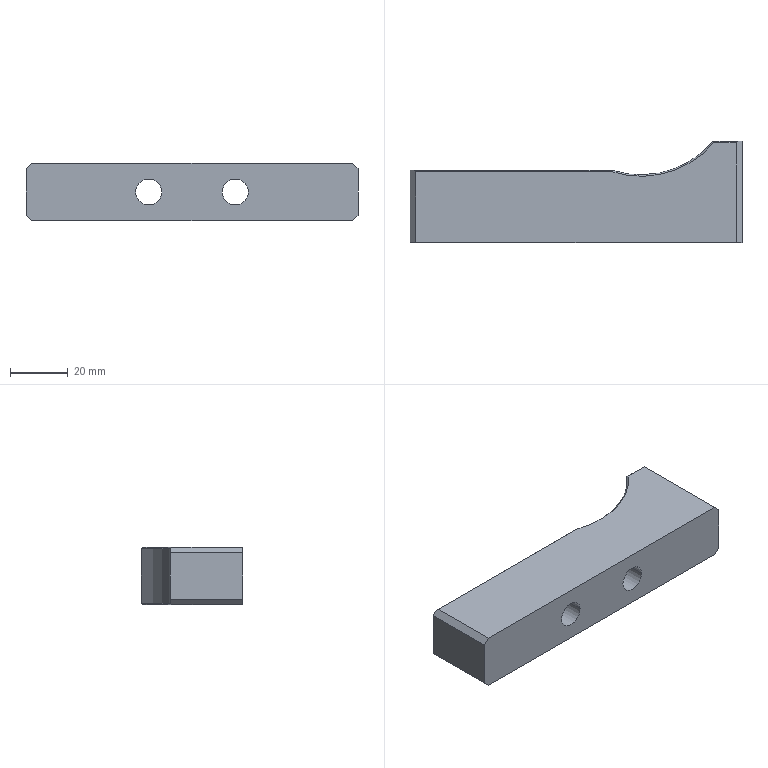Part | SolidWorks | features Chamfer 2, ICE 2, Extrusion 1 | 1 solid | 28 faces | box 115 x 35 x 20 mm | volume 55138 mm3 | plane 17 | cylinder 9 | cone 2 | commonest cylinder face diameters 9 x4 14 x4 65 x1
STEP:
#1=CARTESIAN_POINT('',(77.,0.,10.));
#2=VERTEX_POINT('',#1);
#3=CARTESIAN_POINT('',(68.,0.,10.));
#4=VERTEX_POINT('',#3);
#5=CARTESIAN_POINT('',(72.5,0.,10.));
#6=DIRECTION('',(0.,1.,0.));
#7=DIRECTION('',(-1.,0.,0.));
#8=AXIS2_PLACEMENT_3D('',#5,#6,#7);
#9=CIRCLE('',#8,4.5);
#10=EDGE_CURVE('',#2,#4,#9,.T.);
#11=ORIENTED_EDGE('',*,*,#10,.F.);
#12=CARTESIAN_POINT('',(77.,15.,10.));
#13=VERTEX_POINT('',#12);
#14=CARTESIAN_POINT('',(77.,-5.,10.));
#15=DIRECTION('',(0.,1.,0.));
#16=VECTOR('',#15,1000.);
#17=LINE('',#14,#16);
#18=EDGE_CURVE('',#2,#13,#17,.T.);
#19=ORIENTED_EDGE('',*,*,#18,.T.);
#20=CARTESIAN_POINT('',(68.,15.,10.));
#21=VERTEX_POINT('',#20);
#22=CARTESIAN_POINT('',(72.5,15.,10.));
#23=DIRECTION('',(0.,1.,0.));
#24=DIRECTION('',(-1.,0.,0.));
#25=AXIS2_PLACEMENT_3D('',#22,#23,#24);
#26=CIRCLE('',#25,4.5);
#27=EDGE_CURVE('',#13,#21,#26,.T.);
#28=ORIENTED_EDGE('',*,*,#27,.T.);
#29=CARTESIAN_POINT('',(68.,-5.,10.));
#30=DIRECTION('',(0.,1.,0.));
#31=VECTOR('',#30,1000.);
#32=LINE('',#29,#31);
#33=EDGE_CURVE('',#4,#21,#32,.T.);
#34=ORIENTED_EDGE('',*,*,#33,.F.);
#35=EDGE_LOOP('',(#11,#19,#28,#34));
#36=FACE_OUTER_BOUND('',#35,.T.);
#37=CARTESIAN_POINT('',(72.5,-5.,10.));
#38=DIRECTION('',(0.,1.,0.));
#39=DIRECTION('',(-1.,0.,0.));
#40=AXIS2_PLACEMENT_3D('',#37,#38,#39);
#41=CYLINDRICAL_SURFACE('',#40,4.5);
#42=ADVANCED_FACE('',(#36),#41,.F.);
#43=CARTESIAN_POINT('',(47.,0.,10.));
#44=VERTEX_POINT('',#43);
#45=CARTESIAN_POINT('',(38.,0.,10.));
#46=VERTEX_POINT('',#45);
#47=CARTESIAN_POINT('',(42.5,0.,10.));
#48=DIRECTION('',(0.,1.,0.));
#49=DIRECTION('',(-1.,0.,0.));
#50=AXIS2_PLACEMENT_3D('',#47,#48,#49);
#51=CIRCLE('',#50,4.5);
#52=EDGE_CURVE('',#44,#46,#51,.T.);
#53=ORIENTED_EDGE('',*,*,#52,.F.);
#54=CARTESIAN_POINT('',(47.,15.,10.));
#55=VERTEX_POINT('',#54);
#56=CARTESIAN_POINT('',(47.,-5.,10.));
#57=DIRECTION('',(0.,1.,0.));
#58=VECTOR('',#57,1000.);
#59=LINE('',#56,#58);
#60=EDGE_CURVE('',#44,#55,#59,.T.);
#61=ORIENTED_EDGE('',*,*,#60,.T.);
#62=CARTESIAN_POINT('',(38.,15.,10.));
#63=VERTEX_POINT('',#62);
#64=CARTESIAN_POINT('',(42.5,15.,10.));
#65=DIRECTION('',(0.,1.,0.));
#66=DIRECTION('',(-1.,0.,0.));
#67=AXIS2_PLACEMENT_3D('',#64,#65,#66);
#68=CIRCLE('',#67,4.5);
#69=EDGE_CURVE('',#55,#63,#68,.T.);
#70=ORIENTED_EDGE('',*,*,#69,.T.);
#71=CARTESIAN_POINT('',(38.,-5.,10.));
#72=DIRECTION('',(0.,1.,0.));
#73=VECTOR('',#72,1000.);
#74=LINE('',#71,#73);
#75=EDGE_CURVE('',#46,#63,#74,.T.);
#76=ORIENTED_EDGE('',*,*,#75,.F.);
#77=EDGE_LOOP('',(#53,#61,#70,#76));
#78=FACE_OUTER_BOUND('',#77,.T.);
#79=CARTESIAN_POINT('',(42.5,-5.,10.));
#80=DIRECTION('',(0.,1.,0.));
#81=DIRECTION('',(-1.,0.,0.));
#82=AXIS2_PLACEMENT_3D('',#79,#80,#81);
#83=CYLINDRICAL_SURFACE('',#82,4.5);
#84=ADVANCED_FACE('',(#78),#83,.F.);
#85=CARTESIAN_POINT('',(79.5,15.,10.));
#86=VERTEX_POINT('',#85);
#87=CARTESIAN_POINT('',(65.5,15.,10.));
#88=VERTEX_POINT('',#87);
#89=CARTESIAN_POINT('',(72.5,15.,10.));
#90=DIRECTION('',(0.,1.,0.));
#91=DIRECTION('',(-1.,0.,0.));
#92=AXIS2_PLACEMENT_3D('',#89,#90,#91);
#93=CIRCLE('',#92,7.);
#94=EDGE_CURVE('',#86,#88,#93,.T.);
#95=ORIENTED_EDGE('',*,*,#94,.F.);
#96=CARTESIAN_POINT('',(79.5,23.427,10.));
#97=VERTEX_POINT('',#96);
#98=CARTESIAN_POINT('',(79.5,15.,10.));
#99=DIRECTION('',(0.,1.,0.));
#100=VECTOR('',#99,1000.);
#101=LINE('',#98,#100);
#102=EDGE_CURVE('',#86,#97,#101,.T.);
#103=ORIENTED_EDGE('',*,*,#102,.T.);
#104=CARTESIAN_POINT('',(70.,25.,3.462));
#105=VERTEX_POINT('',#104);
#106=CARTESIAN_POINT('',(70.,25.,3.462));
#107=CARTESIAN_POINT('',(70.255,24.917,3.364));
#108=CARTESIAN_POINT('',(70.52,24.836,3.28));
#109=CARTESIAN_POINT('',(71.054,24.678,3.146));
#110=CARTESIAN_POINT('',(71.323,24.602,3.094));
#111=CARTESIAN_POINT('',(71.867,24.456,3.023));
#112=CARTESIAN_POINT('',(72.142,24.386,3.004));
#113=CARTESIAN_POINT('',(72.697,24.253,2.997));
#114=CARTESIAN_POINT('',(72.978,24.19,3.011));
#115=CARTESIAN_POINT('',(73.815,24.012,3.102));
#116=CARTESIAN_POINT('',(74.36,23.912,3.228));
#117=CARTESIAN_POINT('',(75.156,23.785,3.517));
#118=CARTESIAN_POINT('',(75.419,23.747,3.631));
#119=CARTESIAN_POINT('',(75.926,23.679,3.889));
#120=CARTESIAN_POINT('',(76.17,23.649,4.033));
#121=CARTESIAN_POINT('',(76.64,23.597,4.348));
#122=CARTESIAN_POINT('',(76.866,23.574,4.521));
#123=CARTESIAN_POINT('',(77.298,23.535,4.895));
#124=CARTESIAN_POINT('',(77.505,23.519,5.097));
#125=CARTESIAN_POINT('',(78.078,23.478,5.732));
#126=CARTESIAN_POINT('',(78.405,23.461,6.198));
#127=CARTESIAN_POINT('',(78.948,23.439,7.214));
#128=CARTESIAN_POINT('',(79.152,23.434,7.747));
#129=CARTESIAN_POINT('',(79.36,23.43,8.577));
#130=CARTESIAN_POINT('',(79.413,23.429,8.861));
#131=CARTESIAN_POINT('',(79.483,23.427,9.431));
#132=CARTESIAN_POINT('',(79.5,23.427,9.716));
#133=CARTESIAN_POINT('',(79.5,23.427,10.));
#134=B_SPLINE_CURVE_WITH_KNOTS('',3,(#106,#107,#108,#109,#110,#111,#112,#113,#114,#115,#116,#117,#118,#119,#120,#121,#122,#123,#124,#125,#126,#127,#128,#129,#130,#131,#132,#133),.UNSPECIFIED.,.F.,.F.,(4,2,2,2,2,2,2,2,2,2,2,2,2,4),(0.00863,0.009483,0.01034,0.01119,0.01204,0.01375,0.0146,0.01545,0.01631,0.01716,0.01886,0.02057,0.02142,0.02228),.UNSPECIFIED.);
#135=EDGE_CURVE('',#105,#97,#134,.T.);
#136=ORIENTED_EDGE('',*,*,#135,.F.);
#137=CARTESIAN_POINT('',(65.5,25.,10.));
#138=VERTEX_POINT('',#137);
#139=CARTESIAN_POINT('',(72.5,25.,10.));
#140=DIRECTION('',(0.,-1.,0.));
#141=DIRECTION('',(0.,0.,-1.));
#142=AXIS2_PLACEMENT_3D('',#139,#140,#141);
#143=CIRCLE('',#142,7.);
#144=EDGE_CURVE('',#138,#105,#143,.T.);
#145=ORIENTED_EDGE('',*,*,#144,.F.);
#146=CARTESIAN_POINT('',(65.5,15.,10.));
#147=DIRECTION('',(0.,1.,0.));
#148=VECTOR('',#147,1000.);
#149=LINE('',#146,#148);
#150=EDGE_CURVE('',#88,#138,#149,.T.);
#151=ORIENTED_EDGE('',*,*,#150,.F.);
#152=EDGE_LOOP('',(#95,#103,#136,#145,#151));
#153=FACE_OUTER_BOUND('',#152,.T.);
#154=CARTESIAN_POINT('',(72.5,15.,10.));
#155=DIRECTION('',(0.,1.,0.));
#156=DIRECTION('',(-1.,0.,0.));
#157=AXIS2_PLACEMENT_3D('',#154,#155,#156);
#158=CYLINDRICAL_SURFACE('',#157,7.);
#159=ADVANCED_FACE('',(#153),#158,.F.);
#160=CARTESIAN_POINT('',(49.5,15.,10.));
#161=VERTEX_POINT('',#160);
#162=CARTESIAN_POINT('',(35.5,15.,10.));
#163=VERTEX_POINT('',#162);
#164=CARTESIAN_POINT('',(42.5,15.,10.));
#165=DIRECTION('',(0.,1.,0.));
#166=DIRECTION('',(-1.,0.,0.));
#167=AXIS2_PLACEMENT_3D('',#164,#165,#166);
#168=CIRCLE('',#167,7.);
#169=EDGE_CURVE('',#161,#163,#168,.T.);
#170=ORIENTED_EDGE('',*,*,#169,.F.);
#171=CARTESIAN_POINT('',(49.5,25.,10.));
#172=VERTEX_POINT('',#171);
#173=CARTESIAN_POINT('',(49.5,15.,10.));
#174=DIRECTION('',(0.,1.,0.));
#175=VECTOR('',#174,1000.);
#176=LINE('',#173,#175);
#177=EDGE_CURVE('',#161,#172,#176,.T.);
#178=ORIENTED_EDGE('',*,*,#177,.T.);
#179=CARTESIAN_POINT('',(35.5,25.,10.));
#180=VERTEX_POINT('',#179);
#181=CARTESIAN_POINT('',(42.5,25.,10.));
#182=DIRECTION('',(0.,-1.,0.));
#183=DIRECTION('',(0.,0.,-1.));
#184=AXIS2_PLACEMENT_3D('',#181,#182,#183);
#185=CIRCLE('',#184,7.);
#186=EDGE_CURVE('',#180,#172,#185,.T.);
#187=ORIENTED_EDGE('',*,*,#186,.F.);
#188=CARTESIAN_POINT('',(35.5,15.,10.));
#189=DIRECTION('',(0.,1.,0.));
#190=VECTOR('',#189,1000.);
#191=LINE('',#188,#190);
#192=EDGE_CURVE('',#163,#180,#191,.T.);
#193=ORIENTED_EDGE('',*,*,#192,.F.);
#194=EDGE_LOOP('',(#170,#178,#187,#193));
#195=FACE_OUTER_BOUND('',#194,.T.);
#196=CARTESIAN_POINT('',(42.5,15.,10.));
#197=DIRECTION('',(0.,1.,0.));
#198=DIRECTION('',(-1.,0.,0.));
#199=AXIS2_PLACEMENT_3D('',#196,#197,#198);
#200=CYLINDRICAL_SURFACE('',#199,7.);
#201=ADVANCED_FACE('',(#195),#200,.F.);
#202=CARTESIAN_POINT('',(72.5,0.,10.));
#203=DIRECTION('',(0.,1.,0.));
#204=DIRECTION('',(-1.,0.,0.));
#205=AXIS2_PLACEMENT_3D('',#202,#203,#204);
#206=CIRCLE('',#205,4.5);
#207=EDGE_CURVE('',#4,#2,#206,.T.);
#208=ORIENTED_EDGE('',*,*,#207,.T.);
#209=ORIENTED_EDGE('',*,*,#10,.T.);
#210=EDGE_LOOP('',(#208,#209));
#211=FACE_BOUND('',#210,.T.);
#212=CARTESIAN_POINT('',(42.5,0.,10.));
#213=DIRECTION('',(0.,1.,0.));
#214=DIRECTION('',(-1.,0.,0.));
#215=AXIS2_PLACEMENT_3D('',#212,#213,#214);
#216=CIRCLE('',#215,4.5);
#217=EDGE_CURVE('',#46,#44,#216,.T.);
#218=ORIENTED_EDGE('',*,*,#217,.T.);
#219=ORIENTED_EDGE('',*,*,#52,.T.);
#220=EDGE_LOOP('',(#218,#219));
#221=FACE_BOUND('',#220,.T.);
#222=CARTESIAN_POINT('',(2.,0.,20.));
#223=VERTEX_POINT('',#222);
#224=CARTESIAN_POINT('',(113.,0.,20.));
#225=VERTEX_POINT('',#224);
#226=CARTESIAN_POINT('',(115.,0.,20.));
#227=DIRECTION('',(1.,0.,0.));
#228=VECTOR('',#227,1000.);
#229=LINE('',#226,#228);
#230=EDGE_CURVE('',#223,#225,#229,.T.);
#231=ORIENTED_EDGE('',*,*,#230,.F.);
#232=CARTESIAN_POINT('',(0.,0.,18.));
#233=VERTEX_POINT('',#232);
#234=CARTESIAN_POINT('',(2.,0.,20.));
#235=DIRECTION('',(-0.7071,0.,-0.7071));
#236=VECTOR('',#235,1000.);
#237=LINE('',#234,#236);
#238=EDGE_CURVE('',#223,#233,#237,.T.);
#239=ORIENTED_EDGE('',*,*,#238,.T.);
#240=CARTESIAN_POINT('',(0.,0.,2.));
#241=VERTEX_POINT('',#240);
#242=CARTESIAN_POINT('',(0.,0.,20.));
#243=DIRECTION('',(0.,0.,-1.));
#244=VECTOR('',#243,1000.);
#245=LINE('',#242,#244);
#246=EDGE_CURVE('',#233,#241,#245,.T.);
#247=ORIENTED_EDGE('',*,*,#246,.T.);
#248=CARTESIAN_POINT('',(2.,0.,0.));
#249=VERTEX_POINT('',#248);
#250=CARTESIAN_POINT('',(0.,0.,2.));
#251=DIRECTION('',(0.7071,0.,-0.7071));
#252=VECTOR('',#251,1000.);
#253=LINE('',#250,#252);
#254=EDGE_CURVE('',#241,#249,#253,.T.);
#255=ORIENTED_EDGE('',*,*,#254,.T.);
#256=CARTESIAN_POINT('',(113.,0.,0.));
#257=VERTEX_POINT('',#256);
#258=CARTESIAN_POINT('',(115.,0.,0.));
#259=DIRECTION('',(1.,0.,0.));
#260=VECTOR('',#259,1000.);
#261=LINE('',#258,#260);
#262=EDGE_CURVE('',#249,#257,#261,.T.);
#263=ORIENTED_EDGE('',*,*,#262,.T.);
#264=CARTESIAN_POINT('',(115.,0.,2.));
#265=VERTEX_POINT('',#264);
#266=CARTESIAN_POINT('',(115.,0.,2.));
#267=DIRECTION('',(0.7071,0.,0.7071));
#268=VECTOR('',#267,1000.);
#269=LINE('',#266,#268);
#270=EDGE_CURVE('',#257,#265,#269,.T.);
#271=ORIENTED_EDGE('',*,*,#270,.T.);
#272=CARTESIAN_POINT('',(115.,0.,18.));
#273=VERTEX_POINT('',#272);
#274=CARTESIAN_POINT('',(115.,0.,20.));
#275=DIRECTION('',(0.,0.,-1.));
#276=VECTOR('',#275,1000.);
#277=LINE('',#274,#276);
#278=EDGE_CURVE('',#273,#265,#277,.T.);
#279=ORIENTED_EDGE('',*,*,#278,.F.);
#280=CARTESIAN_POINT('',(113.,0.,20.));
#281=DIRECTION('',(-0.7071,0.,0.7071));
#282=VECTOR('',#281,1000.);
#283=LINE('',#280,#282);
#284=EDGE_CURVE('',#273,#225,#283,.T.);
#285=ORIENTED_EDGE('',*,*,#284,.T.);
#286=EDGE_LOOP('',(#231,#239,#247,#255,#263,#271,#279,#285));
#287=FACE_OUTER_BOUND('',#286,.T.);
#288=CARTESIAN_POINT('',(115.,0.,20.));
#289=DIRECTION('',(0.,1.,0.));
#290=DIRECTION('',(-1.,0.,0.));
#291=AXIS2_PLACEMENT_3D('',#288,#289,#290);
#292=PLANE('',#291);
#293=ADVANCED_FACE('',(#211,#221,#287),#292,.F.);
#294=ORIENTED_EDGE('',*,*,#278,.T.);
#295=CARTESIAN_POINT('',(115.,35.,2.));
#296=VERTEX_POINT('',#295);
#297=CARTESIAN_POINT('',(115.,35.,2.));
#298=DIRECTION('',(0.,1.,0.));
#299=VECTOR('',#298,1000.);
#300=LINE('',#297,#299);
#301=EDGE_CURVE('',#265,#296,#300,.T.);
#302=ORIENTED_EDGE('',*,*,#301,.T.);
#303=CARTESIAN_POINT('',(115.,35.,18.));
#304=VERTEX_POINT('',#303);
#305=CARTESIAN_POINT('',(115.,35.,20.));
#306=DIRECTION('',(0.,0.,-1.));
#307=VECTOR('',#306,1000.);
#308=LINE('',#305,#307);
#309=EDGE_CURVE('',#304,#296,#308,.T.);
#310=ORIENTED_EDGE('',*,*,#309,.F.);
#311=CARTESIAN_POINT('',(115.,0.,18.));
#312=DIRECTION('',(0.,-1.,0.));
#313=VECTOR('',#312,1000.);
#314=LINE('',#311,#313);
#315=EDGE_CURVE('',#304,#273,#314,.T.);
#316=ORIENTED_EDGE('',*,*,#315,.T.);
#317=EDGE_LOOP('',(#294,#302,#310,#316));
#318=FACE_OUTER_BOUND('',#317,.T.);
#319=CARTESIAN_POINT('',(115.,35.,20.));
#320=DIRECTION('',(-1.,0.,0.));
#321=DIRECTION('',(0.,0.,1.));
#322=AXIS2_PLACEMENT_3D('',#319,#320,#321);
#323=PLANE('',#322);
#324=ADVANCED_FACE('',(#318),#323,.F.);
#325=CARTESIAN_POINT('',(113.5,35.,0.5));
#326=VERTEX_POINT('',#325);
#327=CARTESIAN_POINT('',(115.,35.,2.));
#328=DIRECTION('',(-0.7071,0.,-0.7071));
#329=VECTOR('',#328,1000.);
#330=LINE('',#327,#329);
#331=EDGE_CURVE('',#296,#326,#330,.T.);
#332=ORIENTED_EDGE('',*,*,#331,.T.);
#333=CARTESIAN_POINT('',(104.869,35.,0.5));
#334=VERTEX_POINT('',#333);
#335=CARTESIAN_POINT('',(104.869,35.,0.5));
#336=DIRECTION('',(-1.,0.,0.));
#337=VECTOR('',#336,1000.);
#338=LINE('',#335,#337);
#339=EDGE_CURVE('',#326,#334,#338,.T.);
#340=ORIENTED_EDGE('',*,*,#339,.T.);
#341=CARTESIAN_POINT('',(104.869,35.,19.5));
#342=VERTEX_POINT('',#341);
#343=CARTESIAN_POINT('',(104.869,35.,20.));
#344=DIRECTION('',(0.,0.,-1.));
#345=VECTOR('',#344,1000.);
#346=LINE('',#343,#345);
#347=EDGE_CURVE('',#342,#334,#346,.T.);
#348=ORIENTED_EDGE('',*,*,#347,.F.);
#349=CARTESIAN_POINT('',(113.5,35.,19.5));
#350=VERTEX_POINT('',#349);
#351=CARTESIAN_POINT('',(113.,35.,19.5));
#352=DIRECTION('',(1.,0.,0.));
#353=VECTOR('',#352,1000.);
#354=LINE('',#351,#353);
#355=EDGE_CURVE('',#342,#350,#354,.T.);
#356=ORIENTED_EDGE('',*,*,#355,.T.);
#357=CARTESIAN_POINT('',(113.,35.,20.));
#358=DIRECTION('',(0.7071,0.,-0.7071));
#359=VECTOR('',#358,1000.);
#360=LINE('',#357,#359);
#361=EDGE_CURVE('',#350,#304,#360,.T.);
#362=ORIENTED_EDGE('',*,*,#361,.T.);
#363=ORIENTED_EDGE('',*,*,#309,.T.);
#364=EDGE_LOOP('',(#332,#340,#348,#356,#362,#363));
#365=FACE_OUTER_BOUND('',#364,.T.);
#366=CARTESIAN_POINT('',(104.869,35.,20.));
#367=DIRECTION('',(0.,-1.,0.));
#368=DIRECTION('',(0.,0.,-1.));
#369=AXIS2_PLACEMENT_3D('',#366,#367,#368);
#370=PLANE('',#369);
#371=ADVANCED_FACE('',(#365),#370,.F.);
#372=ORIENTED_EDGE('',*,*,#347,.T.);
#373=CARTESIAN_POINT('',(70.,25.,0.5));
#374=VERTEX_POINT('',#373);
#375=CARTESIAN_POINT('',(80.,55.923,0.5));
#376=DIRECTION('',(0.,0.,-1.));
#377=DIRECTION('',(1.,0.,0.));
#378=AXIS2_PLACEMENT_3D('',#375,#376,#377);
#379=CIRCLE('',#378,32.5);
#380=EDGE_CURVE('',#334,#374,#379,.T.);
#381=ORIENTED_EDGE('',*,*,#380,.T.);
#382=CARTESIAN_POINT('',(70.,25.,20.));
#383=DIRECTION('',(0.,0.,-1.));
#384=VECTOR('',#383,1000.);
#385=LINE('',#382,#384);
#386=EDGE_CURVE('',#105,#374,#385,.T.);
#387=ORIENTED_EDGE('',*,*,#386,.F.);
#388=ORIENTED_EDGE('',*,*,#135,.T.);
#389=CARTESIAN_POINT('',(70.,25.,16.538));
#390=VERTEX_POINT('',#389);
#391=CARTESIAN_POINT('',(79.5,23.427,10.));
#392=CARTESIAN_POINT('',(79.5,23.427,10.284));
#393=CARTESIAN_POINT('',(79.483,23.427,10.568));
#394=CARTESIAN_POINT('',(79.413,23.429,11.135));
#395=CARTESIAN_POINT('',(79.36,23.43,11.42));
#396=CARTESIAN_POINT('',(79.152,23.434,12.253));
#397=CARTESIAN_POINT('',(78.948,23.439,12.783));
#398=CARTESIAN_POINT('',(78.544,23.456,13.542));
#399=CARTESIAN_POINT('',(78.393,23.463,13.789));
#400=CARTESIAN_POINT('',(78.065,23.481,14.255));
#401=CARTESIAN_POINT('',(77.888,23.491,14.477));
#402=CARTESIAN_POINT('',(77.317,23.532,15.11));
#403=CARTESIAN_POINT('',(76.878,23.57,15.491));
#404=CARTESIAN_POINT('',(76.173,23.649,15.966));
#405=CARTESIAN_POINT('',(75.929,23.678,16.109));
#406=CARTESIAN_POINT('',(75.425,23.746,16.366));
#407=CARTESIAN_POINT('',(75.163,23.784,16.48));
#408=CARTESIAN_POINT('',(74.362,23.911,16.772));
#409=CARTESIAN_POINT('',(73.817,24.012,16.898));
#410=CARTESIAN_POINT('',(72.983,24.189,16.989));
#411=CARTESIAN_POINT('',(72.7,24.252,17.003));
#412=CARTESIAN_POINT('',(72.144,24.386,16.996));
#413=CARTESIAN_POINT('',(71.869,24.456,16.977));
#414=CARTESIAN_POINT('',(71.324,24.602,16.906));
#415=CARTESIAN_POINT('',(71.054,24.678,16.854));
#416=CARTESIAN_POINT('',(70.519,24.836,16.72));
#417=CARTESIAN_POINT('',(70.255,24.918,16.636));
#418=CARTESIAN_POINT('',(70.,25.,16.538));
#419=B_SPLINE_CURVE_WITH_KNOTS('',3,(#391,#392,#393,#394,#395,#396,#397,#398,#399,#400,#401,#402,#403,#404,#405,#406,#407,#408,#409,#410,#411,#412,#413,#414,#415,#416,#417,#418),.UNSPECIFIED.,.F.,.F.,(4,2,2,2,2,2,2,2,2,2,2,2,2,4),(0.02228,0.02313,0.02398,0.02569,0.02654,0.02739,0.0291,0.02995,0.0308,0.03251,0.03336,0.03421,0.03506,0.03592),.UNSPECIFIED.);
#420=EDGE_CURVE('',#97,#390,#419,.T.);
#421=ORIENTED_EDGE('',*,*,#420,.T.);
#422=CARTESIAN_POINT('',(70.,25.,19.5));
#423=VERTEX_POINT('',#422);
#424=CARTESIAN_POINT('',(70.,25.,20.));
#425=DIRECTION('',(0.,0.,-1.));
#426=VECTOR('',#425,1000.);
#427=LINE('',#424,#426);
#428=EDGE_CURVE('',#423,#390,#427,.T.);
#429=ORIENTED_EDGE('',*,*,#428,.F.);
#430=CARTESIAN_POINT('',(80.,55.923,19.5));
#431=DIRECTION('',(0.,0.,1.));
#432=DIRECTION('',(1.,0.,0.));
#433=AXIS2_PLACEMENT_3D('',#430,#431,#432);
#434=CIRCLE('',#433,32.5);
#435=EDGE_CURVE('',#423,#342,#434,.T.);
#436=ORIENTED_EDGE('',*,*,#435,.T.);
#437=EDGE_LOOP('',(#372,#381,#387,#388,#421,#429,#436));
#438=FACE_OUTER_BOUND('',#437,.T.);
#439=CARTESIAN_POINT('',(80.,55.923,20.));
#440=DIRECTION('',(0.,0.,-1.));
#441=DIRECTION('',(-1.,0.,0.));
#442=AXIS2_PLACEMENT_3D('',#439,#440,#441);
#443=CYLINDRICAL_SURFACE('',#442,32.5);
#444=ADVANCED_FACE('',(#438),#443,.F.);
#445=ORIENTED_EDGE('',*,*,#186,.T.);
#446=CARTESIAN_POINT('',(42.5,25.,10.));
#447=DIRECTION('',(0.,-1.,0.));
#448=DIRECTION('',(0.,0.,-1.));
#449=AXIS2_PLACEMENT_3D('',#446,#447,#448);
#450=CIRCLE('',#449,7.);
#451=EDGE_CURVE('',#172,#180,#450,.T.);
#452=ORIENTED_EDGE('',*,*,#451,.T.);
#453=EDGE_LOOP('',(#445,#452));
#454=FACE_BOUND('',#453,.T.);
#455=ORIENTED_EDGE('',*,*,#386,.T.);
#456=CARTESIAN_POINT('',(1.5,25.,0.5));
#457=VERTEX_POINT('',#456);
#458=CARTESIAN_POINT('',(0.,25.,0.5));
#459=DIRECTION('',(-1.,0.,0.));
#460=VECTOR('',#459,1000.);
#461=LINE('',#458,#460);
#462=EDGE_CURVE('',#374,#457,#461,.T.);
#463=ORIENTED_EDGE('',*,*,#462,.T.);
#464=CARTESIAN_POINT('',(0.,25.,2.));
#465=VERTEX_POINT('',#464);
#466=CARTESIAN_POINT('',(0.,25.,2.));
#467=DIRECTION('',(-0.7071,0.,0.7071));
#468=VECTOR('',#467,1000.);
#469=LINE('',#466,#468);
#470=EDGE_CURVE('',#457,#465,#469,.T.);
#471=ORIENTED_EDGE('',*,*,#470,.T.);
#472=CARTESIAN_POINT('',(0.,25.,18.));
#473=VERTEX_POINT('',#472);
#474=CARTESIAN_POINT('',(0.,25.,20.));
#475=DIRECTION('',(0.,0.,-1.));
#476=VECTOR('',#475,1000.);
#477=LINE('',#474,#476);
#478=EDGE_CURVE('',#473,#465,#477,.T.);
#479=ORIENTED_EDGE('',*,*,#478,.F.);
#480=CARTESIAN_POINT('',(1.5,25.,19.5));
#481=VERTEX_POINT('',#480);
#482=CARTESIAN_POINT('',(2.,25.,20.));
#483=DIRECTION('',(0.7071,0.,0.7071));
#484=VECTOR('',#483,1000.);
#485=LINE('',#482,#484);
#486=EDGE_CURVE('',#473,#481,#485,.T.);
#487=ORIENTED_EDGE('',*,*,#486,.T.);
#488=CARTESIAN_POINT('',(70.,25.,19.5));
#489=DIRECTION('',(1.,0.,0.));
#490=VECTOR('',#489,1000.);
#491=LINE('',#488,#490);
#492=EDGE_CURVE('',#481,#423,#491,.T.);
#493=ORIENTED_EDGE('',*,*,#492,.T.);
#494=ORIENTED_EDGE('',*,*,#428,.T.);
#495=CARTESIAN_POINT('',(72.5,25.,10.));
#496=DIRECTION('',(0.,-1.,0.));
#497=DIRECTION('',(0.,0.,-1.));
#498=AXIS2_PLACEMENT_3D('',#495,#496,#497);
#499=CIRCLE('',#498,7.);
#500=EDGE_CURVE('',#390,#138,#499,.T.);
#501=ORIENTED_EDGE('',*,*,#500,.T.);
#502=ORIENTED_EDGE('',*,*,#144,.T.);
#503=EDGE_LOOP('',(#455,#463,#471,#479,#487,#493,#494,#501,#502));
#504=FACE_OUTER_BOUND('',#503,.T.);
#505=CARTESIAN_POINT('',(0.,25.,20.));
#506=DIRECTION('',(0.,-1.,0.));
#507=DIRECTION('',(0.,0.,-1.));
#508=AXIS2_PLACEMENT_3D('',#505,#506,#507);
#509=PLANE('',#508);
#510=ADVANCED_FACE('',(#454,#504),#509,.F.);
#511=ORIENTED_EDGE('',*,*,#246,.F.);
#512=CARTESIAN_POINT('',(0.,25.,18.));
#513=DIRECTION('',(0.,1.,0.));
#514=VECTOR('',#513,1000.);
#515=LINE('',#512,#514);
#516=EDGE_CURVE('',#233,#473,#515,.T.);
#517=ORIENTED_EDGE('',*,*,#516,.T.);
#518=ORIENTED_EDGE('',*,*,#478,.T.);
#519=CARTESIAN_POINT('',(0.,0.,2.));
#520=DIRECTION('',(0.,-1.,0.));
#521=VECTOR('',#520,1000.);
#522=LINE('',#519,#521);
#523=EDGE_CURVE('',#465,#241,#522,.T.);
#524=ORIENTED_EDGE('',*,*,#523,.T.);
#525=EDGE_LOOP('',(#511,#517,#518,#524));
#526=FACE_OUTER_BOUND('',#525,.T.);
#527=CARTESIAN_POINT('',(0.,0.,20.));
#528=DIRECTION('',(1.,0.,0.));
#529=DIRECTION('',(0.,0.,-1.));
#530=AXIS2_PLACEMENT_3D('',#527,#528,#529);
#531=PLANE('',#530);
#532=ADVANCED_FACE('',(#526),#531,.F.);
#533=CARTESIAN_POINT('',(113.,34.5,20.));
#534=VERTEX_POINT('',#533);
#535=CARTESIAN_POINT('',(113.,35.,20.));
#536=DIRECTION('',(0.,1.,0.));
#537=VECTOR('',#536,1000.);
#538=LINE('',#535,#537);
#539=EDGE_CURVE('',#225,#534,#538,.T.);
#540=ORIENTED_EDGE('',*,*,#539,.T.);
#541=CARTESIAN_POINT('',(105.101,34.5,20.));
#542=VERTEX_POINT('',#541);
#543=CARTESIAN_POINT('',(104.869,34.5,20.));
#544=DIRECTION('',(-1.,0.,0.));
#545=VECTOR('',#544,1000.);
#546=LINE('',#543,#545);
#547=EDGE_CURVE('',#534,#542,#546,.T.);
#548=ORIENTED_EDGE('',*,*,#547,.T.);
#549=CARTESIAN_POINT('',(69.921,24.5,20.));
#550=VERTEX_POINT('',#549);
#551=CARTESIAN_POINT('',(80.,55.923,20.));
#552=DIRECTION('',(0.,0.,-1.));
#553=DIRECTION('',(1.,0.,0.));
#554=AXIS2_PLACEMENT_3D('',#551,#552,#553);
#555=CIRCLE('',#554,33.);
#556=EDGE_CURVE('',#542,#550,#555,.T.);
#557=ORIENTED_EDGE('',*,*,#556,.T.);
#558=CARTESIAN_POINT('',(2.,24.5,20.));
#559=VERTEX_POINT('',#558);
#560=CARTESIAN_POINT('',(2.,24.5,20.));
#561=DIRECTION('',(-1.,0.,0.));
#562=VECTOR('',#561,1000.);
#563=LINE('',#560,#562);
#564=EDGE_CURVE('',#550,#559,#563,.T.);
#565=ORIENTED_EDGE('',*,*,#564,.T.);
#566=CARTESIAN_POINT('',(2.,0.,20.));
#567=DIRECTION('',(0.,-1.,0.));
#568=VECTOR('',#567,1000.);
#569=LINE('',#566,#568);
#570=EDGE_CURVE('',#559,#223,#569,.T.);
#571=ORIENTED_EDGE('',*,*,#570,.T.);
#572=ORIENTED_EDGE('',*,*,#230,.T.);
#573=EDGE_LOOP('',(#540,#548,#557,#565,#571,#572));
#574=FACE_OUTER_BOUND('',#573,.T.);
#575=CARTESIAN_POINT('',(80.,55.923,20.));
#576=DIRECTION('',(0.,0.,1.));
#577=DIRECTION('',(1.,0.,0.));
#578=AXIS2_PLACEMENT_3D('',#575,#576,#577);
#579=PLANE('',#578);
#580=ADVANCED_FACE('',(#574),#579,.T.);
#581=CARTESIAN_POINT('',(69.921,24.5,0.));
#582=VERTEX_POINT('',#581);
#583=CARTESIAN_POINT('',(105.101,34.5,0.));
#584=VERTEX_POINT('',#583);
#585=CARTESIAN_POINT('',(80.,55.923,0.));
#586=DIRECTION('',(0.,0.,1.));
#587=DIRECTION('',(1.,0.,0.));
#588=AXIS2_PLACEMENT_3D('',#585,#586,#587);
#589=CIRCLE('',#588,33.);
#590=EDGE_CURVE('',#582,#584,#589,.T.);
#591=ORIENTED_EDGE('',*,*,#590,.T.);
#592=CARTESIAN_POINT('',(113.,34.5,0.));
#593=VERTEX_POINT('',#592);
#594=CARTESIAN_POINT('',(80.,34.5,0.));
#595=DIRECTION('',(1.,0.,0.));
#596=VECTOR('',#595,1000.);
#597=LINE('',#594,#596);
#598=EDGE_CURVE('',#584,#593,#597,.T.);
#599=ORIENTED_EDGE('',*,*,#598,.T.);
#600=CARTESIAN_POINT('',(113.,55.923,0.));
#601=DIRECTION('',(0.,-1.,0.));
#602=VECTOR('',#601,1000.);
#603=LINE('',#600,#602);
#604=EDGE_CURVE('',#593,#257,#603,.T.);
#605=ORIENTED_EDGE('',*,*,#604,.T.);
#606=ORIENTED_EDGE('',*,*,#262,.F.);
#607=CARTESIAN_POINT('',(2.,24.5,0.));
#608=VERTEX_POINT('',#607);
#609=CARTESIAN_POINT('',(2.,55.923,0.));
#610=DIRECTION('',(0.,1.,0.));
#611=VECTOR('',#610,1000.);
#612=LINE('',#609,#611);
#613=EDGE_CURVE('',#249,#608,#612,.T.);
#614=ORIENTED_EDGE('',*,*,#613,.T.);
#615=CARTESIAN_POINT('',(80.,24.5,0.));
#616=DIRECTION('',(1.,0.,0.));
#617=VECTOR('',#616,1000.);
#618=LINE('',#615,#617);
#619=EDGE_CURVE('',#608,#582,#618,.T.);
#620=ORIENTED_EDGE('',*,*,#619,.T.);
#621=EDGE_LOOP('',(#591,#599,#605,#606,#614,#620));
#622=FACE_OUTER_BOUND('',#621,.T.);
#623=CARTESIAN_POINT('',(80.,55.923,0.));
#624=DIRECTION('',(0.,0.,1.));
#625=DIRECTION('',(1.,0.,0.));
#626=AXIS2_PLACEMENT_3D('',#623,#624,#625);
#627=PLANE('',#626);
#628=ADVANCED_FACE('',(#622),#627,.F.);
#629=ORIENTED_EDGE('',*,*,#177,.F.);
#630=CARTESIAN_POINT('',(42.5,15.,10.));
#631=DIRECTION('',(0.,1.,0.));
#632=DIRECTION('',(-1.,0.,0.));
#633=AXIS2_PLACEMENT_3D('',#630,#631,#632);
#634=CIRCLE('',#633,7.);
#635=EDGE_CURVE('',#163,#161,#634,.T.);
#636=ORIENTED_EDGE('',*,*,#635,.F.);
#637=ORIENTED_EDGE('',*,*,#192,.T.);
#638=ORIENTED_EDGE('',*,*,#451,.F.);
#639=EDGE_LOOP('',(#629,#636,#637,#638));
#640=FACE_OUTER_BOUND('',#639,.T.);
#641=CARTESIAN_POINT('',(42.5,15.,10.));
#642=DIRECTION('',(0.,1.,0.));
#643=DIRECTION('',(-1.,0.,0.));
#644=AXIS2_PLACEMENT_3D('',#641,#642,#643);
#645=CYLINDRICAL_SURFACE('',#644,7.);
#646=ADVANCED_FACE('',(#640),#645,.F.);
#647=CARTESIAN_POINT('',(42.5,15.,10.));
#648=DIRECTION('',(0.,1.,0.));
#649=DIRECTION('',(-1.,0.,0.));
#650=AXIS2_PLACEMENT_3D('',#647,#648,#649);
#651=CIRCLE('',#650,4.5);
#652=EDGE_CURVE('',#63,#55,#651,.T.);
#653=ORIENTED_EDGE('',*,*,#652,.F.);
#654=ORIENTED_EDGE('',*,*,#69,.F.);
#655=EDGE_LOOP('',(#653,#654));
#656=FACE_BOUND('',#655,.T.);
#657=ORIENTED_EDGE('',*,*,#635,.T.);
#658=ORIENTED_EDGE('',*,*,#169,.T.);
#659=EDGE_LOOP('',(#657,#658));
#660=FACE_OUTER_BOUND('',#659,.T.);
#661=CARTESIAN_POINT('',(42.5,15.,10.));
#662=DIRECTION('',(0.,1.,0.));
#663=DIRECTION('',(-1.,0.,0.));
#664=AXIS2_PLACEMENT_3D('',#661,#662,#663);
#665=PLANE('',#664);
#666=ADVANCED_FACE('',(#656,#660),#665,.T.);
#667=ORIENTED_EDGE('',*,*,#102,.F.);
#668=CARTESIAN_POINT('',(72.5,15.,10.));
#669=DIRECTION('',(0.,1.,0.));
#670=DIRECTION('',(-1.,0.,0.));
#671=AXIS2_PLACEMENT_3D('',#668,#669,#670);
#672=CIRCLE('',#671,7.);
#673=EDGE_CURVE('',#88,#86,#672,.T.);
#674=ORIENTED_EDGE('',*,*,#673,.F.);
#675=ORIENTED_EDGE('',*,*,#150,.T.);
#676=ORIENTED_EDGE('',*,*,#500,.F.);
#677=ORIENTED_EDGE('',*,*,#420,.F.);
#678=EDGE_LOOP('',(#667,#674,#675,#676,#677));
#679=FACE_OUTER_BOUND('',#678,.T.);
#680=CARTESIAN_POINT('',(72.5,15.,10.));
#681=DIRECTION('',(0.,1.,0.));
#682=DIRECTION('',(-1.,0.,0.));
#683=AXIS2_PLACEMENT_3D('',#680,#681,#682);
#684=CYLINDRICAL_SURFACE('',#683,7.);
#685=ADVANCED_FACE('',(#679),#684,.F.);
#686=CARTESIAN_POINT('',(72.5,15.,10.));
#687=DIRECTION('',(0.,1.,0.));
#688=DIRECTION('',(-1.,0.,0.));
#689=AXIS2_PLACEMENT_3D('',#686,#687,#688);
#690=CIRCLE('',#689,4.5);
#691=EDGE_CURVE('',#21,#13,#690,.T.);
#692=ORIENTED_EDGE('',*,*,#691,.F.);
#693=ORIENTED_EDGE('',*,*,#27,.F.);
#694=EDGE_LOOP('',(#692,#693));
#695=FACE_BOUND('',#694,.T.);
#696=ORIENTED_EDGE('',*,*,#673,.T.);
#697=ORIENTED_EDGE('',*,*,#94,.T.);
#698=EDGE_LOOP('',(#696,#697));
#699=FACE_OUTER_BOUND('',#698,.T.);
#700=CARTESIAN_POINT('',(72.5,15.,10.));
#701=DIRECTION('',(0.,1.,0.));
#702=DIRECTION('',(-1.,0.,0.));
#703=AXIS2_PLACEMENT_3D('',#700,#701,#702);
#704=PLANE('',#703);
#705=ADVANCED_FACE('',(#695,#699),#704,.T.);
#706=ORIENTED_EDGE('',*,*,#60,.F.);
#707=ORIENTED_EDGE('',*,*,#217,.F.);
#708=ORIENTED_EDGE('',*,*,#75,.T.);
#709=ORIENTED_EDGE('',*,*,#652,.T.);
#710=EDGE_LOOP('',(#706,#707,#708,#709));
#711=FACE_OUTER_BOUND('',#710,.T.);
#712=CARTESIAN_POINT('',(42.5,-5.,10.));
#713=DIRECTION('',(0.,1.,0.));
#714=DIRECTION('',(-1.,0.,0.));
#715=AXIS2_PLACEMENT_3D('',#712,#713,#714);
#716=CYLINDRICAL_SURFACE('',#715,4.5);
#717=ADVANCED_FACE('',(#711),#716,.F.);
#718=ORIENTED_EDGE('',*,*,#18,.F.);
#719=ORIENTED_EDGE('',*,*,#207,.F.);
#720=ORIENTED_EDGE('',*,*,#33,.T.);
#721=ORIENTED_EDGE('',*,*,#691,.T.);
#722=EDGE_LOOP('',(#718,#719,#720,#721));
#723=FACE_OUTER_BOUND('',#722,.T.);
#724=CARTESIAN_POINT('',(72.5,-5.,10.));
#725=DIRECTION('',(0.,1.,0.));
#726=DIRECTION('',(-1.,0.,0.));
#727=AXIS2_PLACEMENT_3D('',#724,#725,#726);
#728=CYLINDRICAL_SURFACE('',#727,4.5);
#729=ADVANCED_FACE('',(#723),#728,.F.);
#730=ORIENTED_EDGE('',*,*,#570,.F.);
#731=CARTESIAN_POINT('',(-8.474,34.974,9.526));
#732=DIRECTION('',(-0.5774,0.5774,-0.5774));
#733=VECTOR('',#732,1000.);
#734=LINE('',#731,#733);
#735=EDGE_CURVE('',#559,#481,#734,.T.);
#736=ORIENTED_EDGE('',*,*,#735,.T.);
#737=ORIENTED_EDGE('',*,*,#486,.F.);
#738=ORIENTED_EDGE('',*,*,#516,.F.);
#739=ORIENTED_EDGE('',*,*,#238,.F.);
#740=EDGE_LOOP('',(#730,#736,#737,#738,#739));
#741=FACE_OUTER_BOUND('',#740,.T.);
#742=CARTESIAN_POINT('',(2.,55.923,20.));
#743=DIRECTION('',(-0.7071,0.,0.7071));
#744=DIRECTION('',(0.,1.,0.));
#745=AXIS2_PLACEMENT_3D('',#742,#743,#744);
#746=PLANE('',#745);
#747=ADVANCED_FACE('',(#741),#746,.T.);
#748=ORIENTED_EDGE('',*,*,#470,.F.);
#749=CARTESIAN_POINT('',(8.833,17.667,-6.833));
#750=DIRECTION('',(0.5774,-0.5774,-0.5774));
#751=VECTOR('',#750,1000.);
#752=LINE('',#749,#751);
#753=EDGE_CURVE('',#457,#608,#752,.T.);
#754=ORIENTED_EDGE('',*,*,#753,.T.);
#755=ORIENTED_EDGE('',*,*,#613,.F.);
#756=ORIENTED_EDGE('',*,*,#254,.F.);
#757=ORIENTED_EDGE('',*,*,#523,.F.);
#758=EDGE_LOOP('',(#748,#754,#755,#756,#757));
#759=FACE_OUTER_BOUND('',#758,.T.);
#760=CARTESIAN_POINT('',(0.,0.,2.));
#761=DIRECTION('',(0.7071,0.,0.7071));
#762=DIRECTION('',(0.,-1.,0.));
#763=AXIS2_PLACEMENT_3D('',#760,#761,#762);
#764=PLANE('',#763);
#765=ADVANCED_FACE('',(#759),#764,.F.);
#766=ORIENTED_EDGE('',*,*,#604,.F.);
#767=CARTESIAN_POINT('',(114.5,36.,1.5));
#768=DIRECTION('',(0.5774,0.5774,0.5774));
#769=VECTOR('',#768,1000.);
#770=LINE('',#767,#769);
#771=EDGE_CURVE('',#593,#326,#770,.T.);
#772=ORIENTED_EDGE('',*,*,#771,.T.);
#773=ORIENTED_EDGE('',*,*,#331,.F.);
#774=ORIENTED_EDGE('',*,*,#301,.F.);
#775=ORIENTED_EDGE('',*,*,#270,.F.);
#776=EDGE_LOOP('',(#766,#772,#773,#774,#775));
#777=FACE_OUTER_BOUND('',#776,.T.);
#778=CARTESIAN_POINT('',(115.,35.,2.));
#779=DIRECTION('',(-0.7071,0.,0.7071));
#780=DIRECTION('',(0.,1.,0.));
#781=AXIS2_PLACEMENT_3D('',#778,#779,#780);
#782=PLANE('',#781);
#783=ADVANCED_FACE('',(#777),#782,.F.);
#784=ORIENTED_EDGE('',*,*,#361,.F.);
#785=CARTESIAN_POINT('',(120.141,41.641,12.859));
#786=DIRECTION('',(-0.5774,-0.5774,0.5774));
#787=VECTOR('',#786,1000.);
#788=LINE('',#785,#787);
#789=EDGE_CURVE('',#350,#534,#788,.T.);
#790=ORIENTED_EDGE('',*,*,#789,.T.);
#791=ORIENTED_EDGE('',*,*,#539,.F.);
#792=ORIENTED_EDGE('',*,*,#284,.F.);
#793=ORIENTED_EDGE('',*,*,#315,.F.);
#794=EDGE_LOOP('',(#784,#790,#791,#792,#793));
#795=FACE_OUTER_BOUND('',#794,.T.);
#796=CARTESIAN_POINT('',(113.,55.923,20.));
#797=DIRECTION('',(0.7071,0.,0.7071));
#798=DIRECTION('',(0.,-1.,0.));
#799=AXIS2_PLACEMENT_3D('',#796,#797,#798);
#800=PLANE('',#799);
#801=ADVANCED_FACE('',(#795),#800,.T.);
#802=ORIENTED_EDGE('',*,*,#753,.F.);
#803=ORIENTED_EDGE('',*,*,#462,.F.);
#804=CARTESIAN_POINT('',(69.921,24.5,0.));
#805=CARTESIAN_POINT('',(69.948,24.667,0.1667));
#806=CARTESIAN_POINT('',(69.974,24.833,0.3333));
#807=CARTESIAN_POINT('',(70.,25.,0.5));
#808=B_SPLINE_CURVE_WITH_KNOTS('',3,(#804,#805,#806,#807),.UNSPECIFIED.,.F.,.F.,(4,4),(0.,0.0007115),.UNSPECIFIED.);
#809=EDGE_CURVE('',#582,#374,#808,.T.);
#810=ORIENTED_EDGE('',*,*,#809,.F.);
#811=ORIENTED_EDGE('',*,*,#619,.F.);
#812=EDGE_LOOP('',(#802,#803,#810,#811));
#813=FACE_OUTER_BOUND('',#812,.T.);
#814=CARTESIAN_POINT('',(0.,25.,0.5));
#815=DIRECTION('',(0.,-0.7071,0.7071));
#816=DIRECTION('',(-1.,0.,0.));
#817=AXIS2_PLACEMENT_3D('',#814,#815,#816);
#818=PLANE('',#817);
#819=ADVANCED_FACE('',(#813),#818,.F.);
#820=ORIENTED_EDGE('',*,*,#809,.T.);
#821=ORIENTED_EDGE('',*,*,#380,.F.);
#822=CARTESIAN_POINT('',(105.101,34.5,0.));
#823=CARTESIAN_POINT('',(105.024,34.667,0.1667));
#824=CARTESIAN_POINT('',(104.947,34.833,0.3334));
#825=CARTESIAN_POINT('',(104.869,35.,0.5));
#826=B_SPLINE_CURVE_WITH_KNOTS('',3,(#822,#823,#824,#825),.UNSPECIFIED.,.F.,.F.,(4,4),(0.,0.0007441),.UNSPECIFIED.);
#827=EDGE_CURVE('',#584,#334,#826,.T.);
#828=ORIENTED_EDGE('',*,*,#827,.F.);
#829=ORIENTED_EDGE('',*,*,#590,.F.);
#830=EDGE_LOOP('',(#820,#821,#828,#829));
#831=FACE_OUTER_BOUND('',#830,.T.);
#832=CARTESIAN_POINT('',(80.,55.923,0.5));
#833=DIRECTION('',(0.,0.,-1.));
#834=DIRECTION('',(-1.,0.,0.));
#835=AXIS2_PLACEMENT_3D('',#832,#833,#834);
#836=CONICAL_SURFACE('',#835,32.5,0.7854);
#837=ADVANCED_FACE('',(#831),#836,.F.);
#838=ORIENTED_EDGE('',*,*,#771,.F.);
#839=ORIENTED_EDGE('',*,*,#598,.F.);
#840=ORIENTED_EDGE('',*,*,#827,.T.);
#841=ORIENTED_EDGE('',*,*,#339,.F.);
#842=EDGE_LOOP('',(#838,#839,#840,#841));
#843=FACE_OUTER_BOUND('',#842,.T.);
#844=CARTESIAN_POINT('',(104.869,35.,0.5));
#845=DIRECTION('',(0.,-0.7071,0.7071));
#846=DIRECTION('',(-1.,0.,0.));
#847=AXIS2_PLACEMENT_3D('',#844,#845,#846);
#848=PLANE('',#847);
#849=ADVANCED_FACE('',(#843),#848,.F.);
#850=ORIENTED_EDGE('',*,*,#735,.F.);
#851=ORIENTED_EDGE('',*,*,#564,.F.);
#852=CARTESIAN_POINT('',(70.,25.,19.5));
#853=CARTESIAN_POINT('',(69.974,24.833,19.667));
#854=CARTESIAN_POINT('',(69.948,24.667,19.833));
#855=CARTESIAN_POINT('',(69.921,24.5,20.));
#856=B_SPLINE_CURVE_WITH_KNOTS('',3,(#852,#853,#854,#855),.UNSPECIFIED.,.F.,.F.,(4,4),(0.,0.0007115),.UNSPECIFIED.);
#857=EDGE_CURVE('',#423,#550,#856,.T.);
#858=ORIENTED_EDGE('',*,*,#857,.F.);
#859=ORIENTED_EDGE('',*,*,#492,.F.);
#860=EDGE_LOOP('',(#850,#851,#858,#859));
#861=FACE_OUTER_BOUND('',#860,.T.);
#862=CARTESIAN_POINT('',(80.,24.5,20.));
#863=DIRECTION('',(0.,0.7071,0.7071));
#864=DIRECTION('',(1.,0.,0.));
#865=AXIS2_PLACEMENT_3D('',#862,#863,#864);
#866=PLANE('',#865);
#867=ADVANCED_FACE('',(#861),#866,.T.);
#868=ORIENTED_EDGE('',*,*,#857,.T.);
#869=ORIENTED_EDGE('',*,*,#556,.F.);
#870=CARTESIAN_POINT('',(104.869,35.,19.5));
#871=CARTESIAN_POINT('',(104.947,34.833,19.667));
#872=CARTESIAN_POINT('',(105.024,34.667,19.833));
#873=CARTESIAN_POINT('',(105.101,34.5,20.));
#874=B_SPLINE_CURVE_WITH_KNOTS('',3,(#870,#871,#872,#873),.UNSPECIFIED.,.F.,.F.,(4,4),(0.,0.0007441),.UNSPECIFIED.);
#875=EDGE_CURVE('',#342,#542,#874,.T.);
#876=ORIENTED_EDGE('',*,*,#875,.F.);
#877=ORIENTED_EDGE('',*,*,#435,.F.);
#878=EDGE_LOOP('',(#868,#869,#876,#877));
#879=FACE_OUTER_BOUND('',#878,.T.);
#880=CARTESIAN_POINT('',(80.,55.923,20.));
#881=DIRECTION('',(0.,0.,1.));
#882=DIRECTION('',(1.,0.,0.));
#883=AXIS2_PLACEMENT_3D('',#880,#881,#882);
#884=CONICAL_SURFACE('',#883,33.,0.7854);
#885=ADVANCED_FACE('',(#879),#884,.F.);
#886=ORIENTED_EDGE('',*,*,#789,.F.);
#887=ORIENTED_EDGE('',*,*,#355,.F.);
#888=ORIENTED_EDGE('',*,*,#875,.T.);
#889=ORIENTED_EDGE('',*,*,#547,.F.);
#890=EDGE_LOOP('',(#886,#887,#888,#889));
#891=FACE_OUTER_BOUND('',#890,.T.);
#892=CARTESIAN_POINT('',(80.,34.5,20.));
#893=DIRECTION('',(0.,0.7071,0.7071));
#894=DIRECTION('',(1.,0.,0.));
#895=AXIS2_PLACEMENT_3D('',#892,#893,#894);
#896=PLANE('',#895);
#897=ADVANCED_FACE('',(#891),#896,.T.);
#898=CLOSED_SHELL('',(#42,#84,#159,#201,#293,#324,#371,#444,#510,#532,#580,#628,#646,#666,#685,#705,#717,#729,#747,#765,#783,#801,#819,#837,#849,#867,#885,#897));
#899=MANIFOLD_SOLID_BREP('',#898);
#900=CARTESIAN_POINT('',(0.,0.,0.));
#901=DIRECTION('',(0.,0.,1.));
#902=DIRECTION('',(1.,0.,0.));
#903=AXIS2_PLACEMENT_3D('',#900,#901,#902);
#904=(LENGTH_UNIT()NAMED_UNIT(*)SI_UNIT(.MILLI.,.METRE.));
#905=UNCERTAINTY_MEASURE_WITH_UNIT(LENGTH_MEASURE(0.00001),#904,'','');
#906=(NAMED_UNIT(*)PLANE_ANGLE_UNIT()SI_UNIT($,.RADIAN.));
#907=(NAMED_UNIT(*)SI_UNIT($,.STERADIAN.)SOLID_ANGLE_UNIT());
#908=(GEOMETRIC_REPRESENTATION_CONTEXT(3)GLOBAL_UNCERTAINTY_ASSIGNED_CONTEXT((#905))GLOBAL_UNIT_ASSIGNED_CONTEXT((#904,#906,#907))REPRESENTATION_CONTEXT('',''));
#909=ADVANCED_BREP_SHAPE_REPRESENTATION('',(#899,#903),#908);